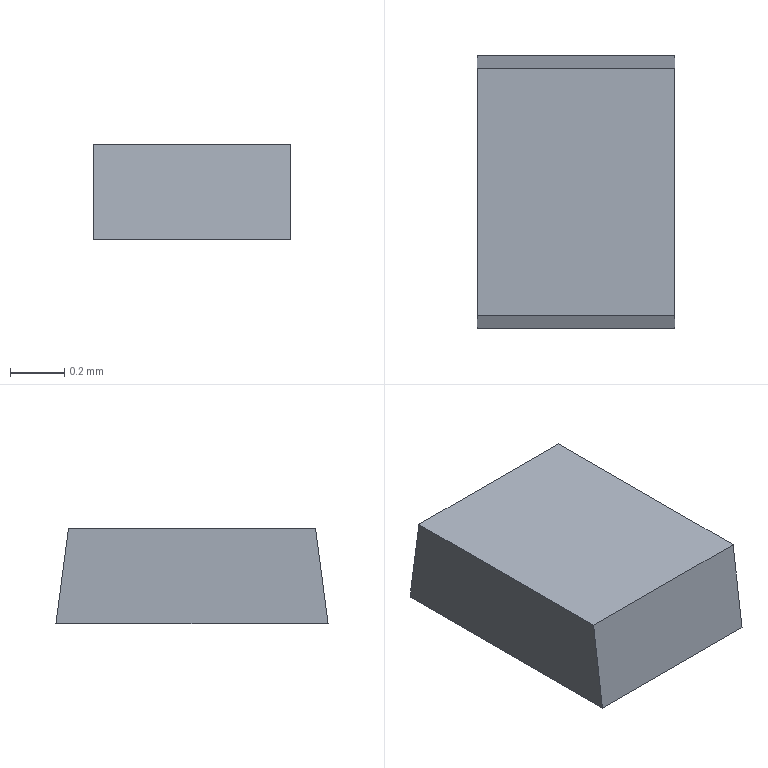Part | STEP file | RJ-USIO-V1_2-220411_177 | 1 solid | 6 faces | box 0.725 x 1 x 0.35 mm | volume 0.242 mm3 | plane 6
STEP:
#1=CARTESIAN_POINT('',(0.,0.,0.));
#2=DIRECTION('',(0.,0.,1.));
#3=DIRECTION('',(1.,0.,0.));
#4=AXIS2_PLACEMENT_3D('',#1,#2,#3);
#5=CARTESIAN_POINT('',(60.862,67.4,0.3298));
#6=VERTEX_POINT('',#5);
#7=CARTESIAN_POINT('',(60.862,66.4,0.3298));
#8=VERTEX_POINT('',#7);
#9=CARTESIAN_POINT('',(60.862,67.4,0.3298));
#10=DIRECTION('',(0.000000175,-1.,0.));
#11=VECTOR('',#10,1.);
#12=LINE('',#9,#11);
#13=CARTESIAN_POINT('',(60.5,66.9,0.3298));
#14=DIRECTION('',(0.,0.,1.));
#15=DIRECTION('',(-1.,-0.000000175,0.));
#16=AXIS2_PLACEMENT_3D('',#13,#14,#15);
#17=PLANE('',#16);
#18=CARTESIAN_POINT('',(-0.3625,-0.5));
#19=DIRECTION('',(0.,1.));
#20=VECTOR('',#19,1.);
#21=LINE('',#18,#20);
#22=(GEOMETRIC_REPRESENTATION_CONTEXT(2)PARAMETRIC_REPRESENTATION_CONTEXT()REPRESENTATION_CONTEXT('',''));
#23=DEFINITIONAL_REPRESENTATION('',(#21),#22);
#24=PCURVE('',#17,#23);
#25=CARTESIAN_POINT('',(60.862,66.4,0.3298));
#26=DIRECTION('',(1.,0.000000175,0.));
#27=DIRECTION('',(0.000000175,-1.,0.));
#28=AXIS2_PLACEMENT_3D('',#25,#26,#27);
#29=PLANE('',#28);
#30=CARTESIAN_POINT('',(-1.,0.));
#31=DIRECTION('',(1.,0.));
#32=VECTOR('',#31,1.);
#33=LINE('',#30,#32);
#34=(GEOMETRIC_REPRESENTATION_CONTEXT(2)PARAMETRIC_REPRESENTATION_CONTEXT()REPRESENTATION_CONTEXT('',''));
#35=DEFINITIONAL_REPRESENTATION('',(#33),#34);
#36=PCURVE('',#29,#35);
#37=SURFACE_CURVE('',#12,(#24,#36),.PCURVE_S1.);
#38=EDGE_CURVE('',#6,#8,#37,.T.);
#39=ORIENTED_EDGE('',*,*,#38,.F.);
#40=CARTESIAN_POINT('',(60.137,67.4,0.3298));
#41=VERTEX_POINT('',#40);
#42=CARTESIAN_POINT('',(60.137,67.4,0.3298));
#43=DIRECTION('',(1.,0.000000175,0.));
#44=VECTOR('',#43,1.);
#45=LINE('',#42,#44);
#46=CARTESIAN_POINT('',(0.3625,-0.5));
#47=DIRECTION('',(-1.,0.));
#48=VECTOR('',#47,1.);
#49=LINE('',#46,#48);
#50=(GEOMETRIC_REPRESENTATION_CONTEXT(2)PARAMETRIC_REPRESENTATION_CONTEXT()REPRESENTATION_CONTEXT('',''));
#51=DEFINITIONAL_REPRESENTATION('',(#49),#50);
#52=PCURVE('',#17,#51);
#53=CARTESIAN_POINT('',(60.681,67.377,0.5048));
#54=DIRECTION('',(-0.000000173,0.9914,0.1309));
#55=DIRECTION('',(-0.000000023,0.1309,-0.9914));
#56=AXIS2_PLACEMENT_3D('',#53,#54,#55);
#57=PLANE('',#56);
#58=CARTESIAN_POINT('',(0.1765,0.5438));
#59=DIRECTION('',(0.,-1.));
#60=VECTOR('',#59,1.);
#61=LINE('',#58,#60);
#62=(GEOMETRIC_REPRESENTATION_CONTEXT(2)PARAMETRIC_REPRESENTATION_CONTEXT()REPRESENTATION_CONTEXT('',''));
#63=DEFINITIONAL_REPRESENTATION('',(#61),#62);
#64=PCURVE('',#57,#63);
#65=SURFACE_CURVE('',#45,(#52,#64),.PCURVE_S1.);
#66=EDGE_CURVE('',#41,#6,#65,.T.);
#67=ORIENTED_EDGE('',*,*,#66,.F.);
#68=CARTESIAN_POINT('',(60.137,66.4,0.3298));
#69=VERTEX_POINT('',#68);
#70=CARTESIAN_POINT('',(60.137,66.4,0.3298));
#71=DIRECTION('',(-0.000000175,1.,0.));
#72=VECTOR('',#71,1.);
#73=LINE('',#70,#72);
#74=CARTESIAN_POINT('',(0.3625,0.5));
#75=DIRECTION('',(0.,-1.));
#76=VECTOR('',#75,1.);
#77=LINE('',#74,#76);
#78=(GEOMETRIC_REPRESENTATION_CONTEXT(2)PARAMETRIC_REPRESENTATION_CONTEXT()REPRESENTATION_CONTEXT('',''));
#79=DEFINITIONAL_REPRESENTATION('',(#77),#78);
#80=PCURVE('',#17,#79);
#81=CARTESIAN_POINT('',(60.137,67.4,0.3298));
#82=DIRECTION('',(-1.,-0.000000175,0.));
#83=DIRECTION('',(-0.000000175,1.,0.));
#84=AXIS2_PLACEMENT_3D('',#81,#82,#83);
#85=PLANE('',#84);
#86=CARTESIAN_POINT('',(-1.,0.));
#87=DIRECTION('',(1.,0.));
#88=VECTOR('',#87,1.);
#89=LINE('',#86,#88);
#90=(GEOMETRIC_REPRESENTATION_CONTEXT(2)PARAMETRIC_REPRESENTATION_CONTEXT()REPRESENTATION_CONTEXT('',''));
#91=DEFINITIONAL_REPRESENTATION('',(#89),#90);
#92=PCURVE('',#85,#91);
#93=SURFACE_CURVE('',#73,(#80,#92),.PCURVE_S1.);
#94=EDGE_CURVE('',#69,#41,#93,.T.);
#95=ORIENTED_EDGE('',*,*,#94,.F.);
#96=CARTESIAN_POINT('',(60.862,66.4,0.3298));
#97=DIRECTION('',(-1.,-0.000000175,0.));
#98=VECTOR('',#97,1.);
#99=LINE('',#96,#98);
#100=CARTESIAN_POINT('',(-0.3625,0.5));
#101=DIRECTION('',(1.,0.));
#102=VECTOR('',#101,1.);
#103=LINE('',#100,#102);
#104=(GEOMETRIC_REPRESENTATION_CONTEXT(2)PARAMETRIC_REPRESENTATION_CONTEXT()REPRESENTATION_CONTEXT('',''));
#105=DEFINITIONAL_REPRESENTATION('',(#103),#104);
#106=PCURVE('',#17,#105);
#107=CARTESIAN_POINT('',(60.681,66.423,0.5048));
#108=DIRECTION('',(0.000000173,-0.9914,0.1309));
#109=DIRECTION('',(-0.000000023,0.1309,0.9914));
#110=AXIS2_PLACEMENT_3D('',#107,#108,#109);
#111=PLANE('',#110);
#112=CARTESIAN_POINT('',(-0.1765,-0.1813));
#113=DIRECTION('',(0.,1.));
#114=VECTOR('',#113,1.);
#115=LINE('',#112,#114);
#116=(GEOMETRIC_REPRESENTATION_CONTEXT(2)PARAMETRIC_REPRESENTATION_CONTEXT()REPRESENTATION_CONTEXT('',''));
#117=DEFINITIONAL_REPRESENTATION('',(#115),#116);
#118=PCURVE('',#111,#117);
#119=SURFACE_CURVE('',#99,(#106,#118),.PCURVE_S1.);
#120=EDGE_CURVE('',#8,#69,#119,.T.);
#121=ORIENTED_EDGE('',*,*,#120,.F.);
#122=EDGE_LOOP('',(#39,#67,#95,#121));
#123=FACE_BOUND('',#122,.F.);
#124=ADVANCED_FACE('',(#123),#17,.F.);
#125=ORIENTED_EDGE('',*,*,#38,.T.);
#126=CARTESIAN_POINT('',(60.862,66.446,0.6798));
#127=VERTEX_POINT('',#126);
#128=CARTESIAN_POINT('',(60.862,66.446,0.6798));
#129=DIRECTION('',(0.000000023,-0.1309,-0.9914));
#130=VECTOR('',#129,1.);
#131=LINE('',#128,#130);
#132=CARTESIAN_POINT('',(-0.0462,-0.35));
#133=DIRECTION('',(0.1309,0.9914));
#134=VECTOR('',#133,1.);
#135=LINE('',#132,#134);
#136=(GEOMETRIC_REPRESENTATION_CONTEXT(2)PARAMETRIC_REPRESENTATION_CONTEXT()REPRESENTATION_CONTEXT('',''));
#137=DEFINITIONAL_REPRESENTATION('',(#135),#136);
#138=PCURVE('',#29,#137);
#139=CARTESIAN_POINT('',(0.1765,-0.1812));
#140=DIRECTION('',(-1.,0.));
#141=VECTOR('',#140,1.);
#142=LINE('',#139,#141);
#143=(GEOMETRIC_REPRESENTATION_CONTEXT(2)PARAMETRIC_REPRESENTATION_CONTEXT()REPRESENTATION_CONTEXT('',''));
#144=DEFINITIONAL_REPRESENTATION('',(#142),#143);
#145=PCURVE('',#111,#144);
#146=SURFACE_CURVE('',#131,(#138,#145),.PCURVE_S1.);
#147=EDGE_CURVE('',#127,#8,#146,.T.);
#148=ORIENTED_EDGE('',*,*,#147,.F.);
#149=CARTESIAN_POINT('',(60.862,67.354,0.6798));
#150=VERTEX_POINT('',#149);
#151=CARTESIAN_POINT('',(60.862,66.446,0.6798));
#152=DIRECTION('',(-0.000000175,1.,0.));
#153=VECTOR('',#152,1.);
#154=LINE('',#151,#153);
#155=CARTESIAN_POINT('',(-0.0462,-0.35));
#156=DIRECTION('',(-1.,0.));
#157=VECTOR('',#156,1.);
#158=LINE('',#155,#157);
#159=(GEOMETRIC_REPRESENTATION_CONTEXT(2)PARAMETRIC_REPRESENTATION_CONTEXT()REPRESENTATION_CONTEXT('',''));
#160=DEFINITIONAL_REPRESENTATION('',(#158),#159);
#161=PCURVE('',#29,#160);
#162=CARTESIAN_POINT('',(60.5,66.9,0.6798));
#163=DIRECTION('',(0.,0.,1.));
#164=DIRECTION('',(-1.,-0.000000175,0.));
#165=AXIS2_PLACEMENT_3D('',#162,#163,#164);
#166=PLANE('',#165);
#167=CARTESIAN_POINT('',(-0.3625,0.4538));
#168=DIRECTION('',(0.,-1.));
#169=VECTOR('',#168,1.);
#170=LINE('',#167,#169);
#171=(GEOMETRIC_REPRESENTATION_CONTEXT(2)PARAMETRIC_REPRESENTATION_CONTEXT()REPRESENTATION_CONTEXT('',''));
#172=DEFINITIONAL_REPRESENTATION('',(#170),#171);
#173=PCURVE('',#166,#172);
#174=SURFACE_CURVE('',#154,(#161,#173),.PCURVE_S1.);
#175=EDGE_CURVE('',#127,#150,#174,.T.);
#176=ORIENTED_EDGE('',*,*,#175,.T.);
#177=CARTESIAN_POINT('',(60.862,67.4,0.3298));
#178=DIRECTION('',(0.000000023,-0.1309,0.9914));
#179=VECTOR('',#178,1.);
#180=LINE('',#177,#179);
#181=CARTESIAN_POINT('',(-1.,0.));
#182=DIRECTION('',(0.1309,-0.9914));
#183=VECTOR('',#182,1.);
#184=LINE('',#181,#183);
#185=(GEOMETRIC_REPRESENTATION_CONTEXT(2)PARAMETRIC_REPRESENTATION_CONTEXT()REPRESENTATION_CONTEXT('',''));
#186=DEFINITIONAL_REPRESENTATION('',(#184),#185);
#187=PCURVE('',#29,#186);
#188=CARTESIAN_POINT('',(0.1765,-0.1812));
#189=DIRECTION('',(-1.,0.));
#190=VECTOR('',#189,1.);
#191=LINE('',#188,#190);
#192=(GEOMETRIC_REPRESENTATION_CONTEXT(2)PARAMETRIC_REPRESENTATION_CONTEXT()REPRESENTATION_CONTEXT('',''));
#193=DEFINITIONAL_REPRESENTATION('',(#191),#192);
#194=PCURVE('',#57,#193);
#195=SURFACE_CURVE('',#180,(#187,#194),.PCURVE_S1.);
#196=EDGE_CURVE('',#6,#150,#195,.T.);
#197=ORIENTED_EDGE('',*,*,#196,.F.);
#198=EDGE_LOOP('',(#125,#148,#176,#197));
#199=FACE_BOUND('',#198,.F.);
#200=ADVANCED_FACE('',(#199),#29,.T.);
#201=CARTESIAN_POINT('',(60.137,66.446,0.6798));
#202=VERTEX_POINT('',#201);
#203=CARTESIAN_POINT('',(60.137,66.4,0.3298));
#204=DIRECTION('',(-0.000000023,0.1309,0.9914));
#205=VECTOR('',#204,1.);
#206=LINE('',#203,#205);
#207=CARTESIAN_POINT('',(-0.1765,0.5437));
#208=DIRECTION('',(1.,0.));
#209=VECTOR('',#208,1.);
#210=LINE('',#207,#209);
#211=(GEOMETRIC_REPRESENTATION_CONTEXT(2)PARAMETRIC_REPRESENTATION_CONTEXT()REPRESENTATION_CONTEXT('',''));
#212=DEFINITIONAL_REPRESENTATION('',(#210),#211);
#213=PCURVE('',#111,#212);
#214=CARTESIAN_POINT('',(-1.,0.));
#215=DIRECTION('',(0.1309,-0.9914));
#216=VECTOR('',#215,1.);
#217=LINE('',#214,#216);
#218=(GEOMETRIC_REPRESENTATION_CONTEXT(2)PARAMETRIC_REPRESENTATION_CONTEXT()REPRESENTATION_CONTEXT('',''));
#219=DEFINITIONAL_REPRESENTATION('',(#217),#218);
#220=PCURVE('',#85,#219);
#221=SURFACE_CURVE('',#206,(#213,#220),.PCURVE_S1.);
#222=EDGE_CURVE('',#69,#202,#221,.T.);
#223=ORIENTED_EDGE('',*,*,#222,.T.);
#224=CARTESIAN_POINT('',(60.137,66.446,0.6798));
#225=DIRECTION('',(1.,0.000000175,0.));
#226=VECTOR('',#225,1.);
#227=LINE('',#224,#226);
#228=CARTESIAN_POINT('',(0.1765,0.5438));
#229=DIRECTION('',(0.,-1.));
#230=VECTOR('',#229,1.);
#231=LINE('',#228,#230);
#232=(GEOMETRIC_REPRESENTATION_CONTEXT(2)PARAMETRIC_REPRESENTATION_CONTEXT()REPRESENTATION_CONTEXT('',''));
#233=DEFINITIONAL_REPRESENTATION('',(#231),#232);
#234=PCURVE('',#111,#233);
#235=CARTESIAN_POINT('',(0.3625,0.4538));
#236=DIRECTION('',(-1.,0.));
#237=VECTOR('',#236,1.);
#238=LINE('',#235,#237);
#239=(GEOMETRIC_REPRESENTATION_CONTEXT(2)PARAMETRIC_REPRESENTATION_CONTEXT()REPRESENTATION_CONTEXT('',''));
#240=DEFINITIONAL_REPRESENTATION('',(#238),#239);
#241=PCURVE('',#166,#240);
#242=SURFACE_CURVE('',#227,(#234,#241),.PCURVE_S1.);
#243=EDGE_CURVE('',#202,#127,#242,.T.);
#244=ORIENTED_EDGE('',*,*,#243,.T.);
#245=ORIENTED_EDGE('',*,*,#147,.T.);
#246=ORIENTED_EDGE('',*,*,#120,.T.);
#247=EDGE_LOOP('',(#223,#244,#245,#246));
#248=FACE_BOUND('',#247,.F.);
#249=ADVANCED_FACE('',(#248),#111,.T.);
#250=CARTESIAN_POINT('',(60.137,67.354,0.6798));
#251=VERTEX_POINT('',#250);
#252=CARTESIAN_POINT('',(60.137,67.354,0.6798));
#253=DIRECTION('',(0.000000175,-1.,0.));
#254=VECTOR('',#253,1.);
#255=LINE('',#252,#254);
#256=CARTESIAN_POINT('',(-0.0462,-0.35));
#257=DIRECTION('',(-1.,0.));
#258=VECTOR('',#257,1.);
#259=LINE('',#256,#258);
#260=(GEOMETRIC_REPRESENTATION_CONTEXT(2)PARAMETRIC_REPRESENTATION_CONTEXT()REPRESENTATION_CONTEXT('',''));
#261=DEFINITIONAL_REPRESENTATION('',(#259),#260);
#262=PCURVE('',#85,#261);
#263=CARTESIAN_POINT('',(0.3625,-0.4538));
#264=DIRECTION('',(0.,1.));
#265=VECTOR('',#264,1.);
#266=LINE('',#263,#265);
#267=(GEOMETRIC_REPRESENTATION_CONTEXT(2)PARAMETRIC_REPRESENTATION_CONTEXT()REPRESENTATION_CONTEXT('',''));
#268=DEFINITIONAL_REPRESENTATION('',(#266),#267);
#269=PCURVE('',#166,#268);
#270=SURFACE_CURVE('',#255,(#262,#269),.PCURVE_S1.);
#271=EDGE_CURVE('',#251,#202,#270,.T.);
#272=ORIENTED_EDGE('',*,*,#271,.T.);
#273=ORIENTED_EDGE('',*,*,#222,.F.);
#274=ORIENTED_EDGE('',*,*,#94,.T.);
#275=CARTESIAN_POINT('',(60.137,67.354,0.6798));
#276=DIRECTION('',(-0.000000023,0.1309,-0.9914));
#277=VECTOR('',#276,1.);
#278=LINE('',#275,#277);
#279=CARTESIAN_POINT('',(-0.0462,-0.35));
#280=DIRECTION('',(0.1309,0.9914));
#281=VECTOR('',#280,1.);
#282=LINE('',#279,#281);
#283=(GEOMETRIC_REPRESENTATION_CONTEXT(2)PARAMETRIC_REPRESENTATION_CONTEXT()REPRESENTATION_CONTEXT('',''));
#284=DEFINITIONAL_REPRESENTATION('',(#282),#283);
#285=PCURVE('',#85,#284);
#286=CARTESIAN_POINT('',(-0.1765,0.5438));
#287=DIRECTION('',(1.,0.));
#288=VECTOR('',#287,1.);
#289=LINE('',#286,#288);
#290=(GEOMETRIC_REPRESENTATION_CONTEXT(2)PARAMETRIC_REPRESENTATION_CONTEXT()REPRESENTATION_CONTEXT('',''));
#291=DEFINITIONAL_REPRESENTATION('',(#289),#290);
#292=PCURVE('',#57,#291);
#293=SURFACE_CURVE('',#278,(#285,#292),.PCURVE_S1.);
#294=EDGE_CURVE('',#251,#41,#293,.T.);
#295=ORIENTED_EDGE('',*,*,#294,.F.);
#296=EDGE_LOOP('',(#272,#273,#274,#295));
#297=FACE_BOUND('',#296,.F.);
#298=ADVANCED_FACE('',(#297),#85,.T.);
#299=ORIENTED_EDGE('',*,*,#175,.F.);
#300=ORIENTED_EDGE('',*,*,#243,.F.);
#301=ORIENTED_EDGE('',*,*,#271,.F.);
#302=CARTESIAN_POINT('',(60.862,67.354,0.6798));
#303=DIRECTION('',(-1.,-0.000000175,0.));
#304=VECTOR('',#303,1.);
#305=LINE('',#302,#304);
#306=CARTESIAN_POINT('',(-0.3625,-0.4538));
#307=DIRECTION('',(1.,0.));
#308=VECTOR('',#307,1.);
#309=LINE('',#306,#308);
#310=(GEOMETRIC_REPRESENTATION_CONTEXT(2)PARAMETRIC_REPRESENTATION_CONTEXT()REPRESENTATION_CONTEXT('',''));
#311=DEFINITIONAL_REPRESENTATION('',(#309),#310);
#312=PCURVE('',#166,#311);
#313=CARTESIAN_POINT('',(-0.1765,-0.1812));
#314=DIRECTION('',(0.,1.));
#315=VECTOR('',#314,1.);
#316=LINE('',#313,#315);
#317=(GEOMETRIC_REPRESENTATION_CONTEXT(2)PARAMETRIC_REPRESENTATION_CONTEXT()REPRESENTATION_CONTEXT('',''));
#318=DEFINITIONAL_REPRESENTATION('',(#316),#317);
#319=PCURVE('',#57,#318);
#320=SURFACE_CURVE('',#305,(#312,#319),.PCURVE_S1.);
#321=EDGE_CURVE('',#150,#251,#320,.T.);
#322=ORIENTED_EDGE('',*,*,#321,.F.);
#323=EDGE_LOOP('',(#299,#300,#301,#322));
#324=FACE_BOUND('',#323,.F.);
#325=ADVANCED_FACE('',(#324),#166,.T.);
#326=ORIENTED_EDGE('',*,*,#294,.T.);
#327=ORIENTED_EDGE('',*,*,#66,.T.);
#328=ORIENTED_EDGE('',*,*,#196,.T.);
#329=ORIENTED_EDGE('',*,*,#321,.T.);
#330=EDGE_LOOP('',(#326,#327,#328,#329));
#331=FACE_BOUND('',#330,.F.);
#332=ADVANCED_FACE('',(#331),#57,.T.);
#333=CLOSED_SHELL('',(#124,#200,#249,#298,#325,#332));
#334=MANIFOLD_SOLID_BREP('',#333);
#335=(LENGTH_UNIT()NAMED_UNIT(*)SI_UNIT(.MILLI.,.METRE.));
#336=UNCERTAINTY_MEASURE_WITH_UNIT(LENGTH_MEASURE(0.0000001),#335,'','');
#337=(NAMED_UNIT(*)PLANE_ANGLE_UNIT()SI_UNIT($,.RADIAN.));
#338=(NAMED_UNIT(*)SI_UNIT($,.STERADIAN.)SOLID_ANGLE_UNIT());
#339=(GEOMETRIC_REPRESENTATION_CONTEXT(3)GLOBAL_UNCERTAINTY_ASSIGNED_CONTEXT((#336))GLOBAL_UNIT_ASSIGNED_CONTEXT((#335,#337,#338))REPRESENTATION_CONTEXT('',''));
#340=ADVANCED_BREP_SHAPE_REPRESENTATION('',(#4,#334),#339);